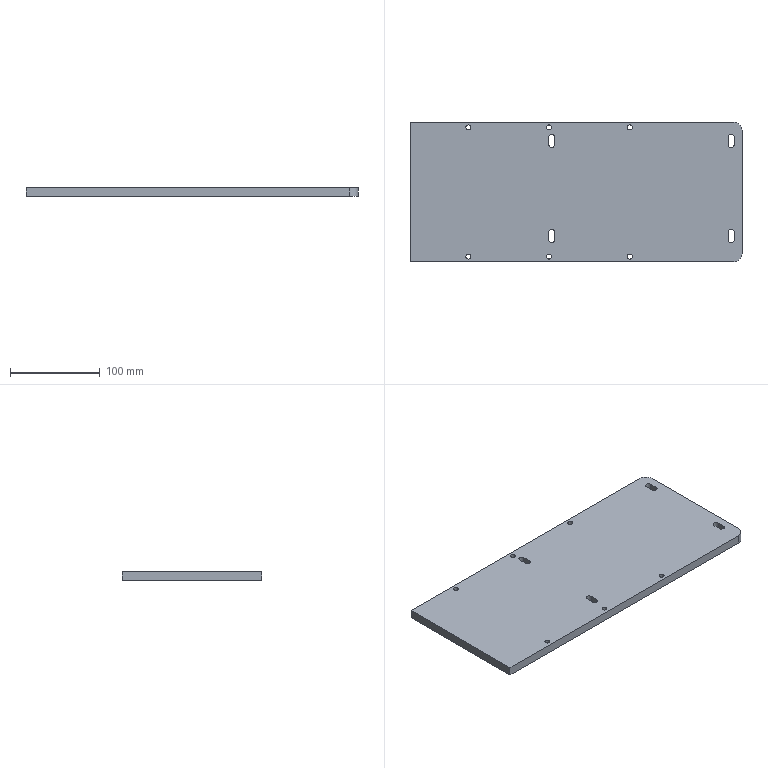Part | STEP file | FBDS-BEI | 1 solid | 54 faces | box 370 x 156 x 10 mm | volume 569992 mm3 | cylinder 34 | plane 20 | commonest cylinder face diameters 5.5 x12 9.8 x12 6.6 x8 20 x2